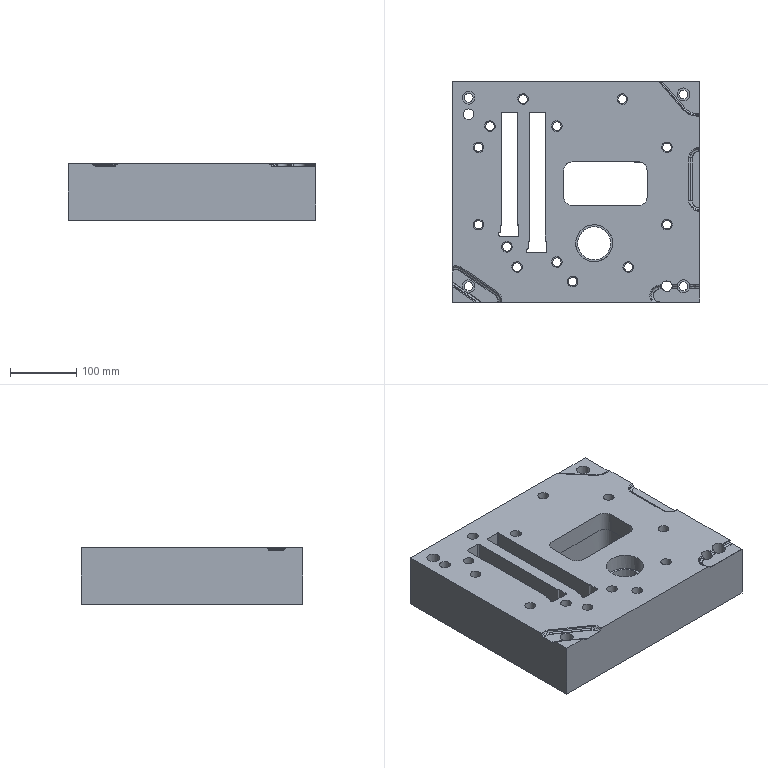Part | NX | features solid 2 | 1 solid | 145 faces | box 375.001 x 335.008 x 85 mm | volume 8526263 mm3 | spline 78 | cylinder 38 | plane 29 | commonest cylinder face diameters 16 x15 13 x13 13.5 x4 19.5 x4 50 x1 56 x1